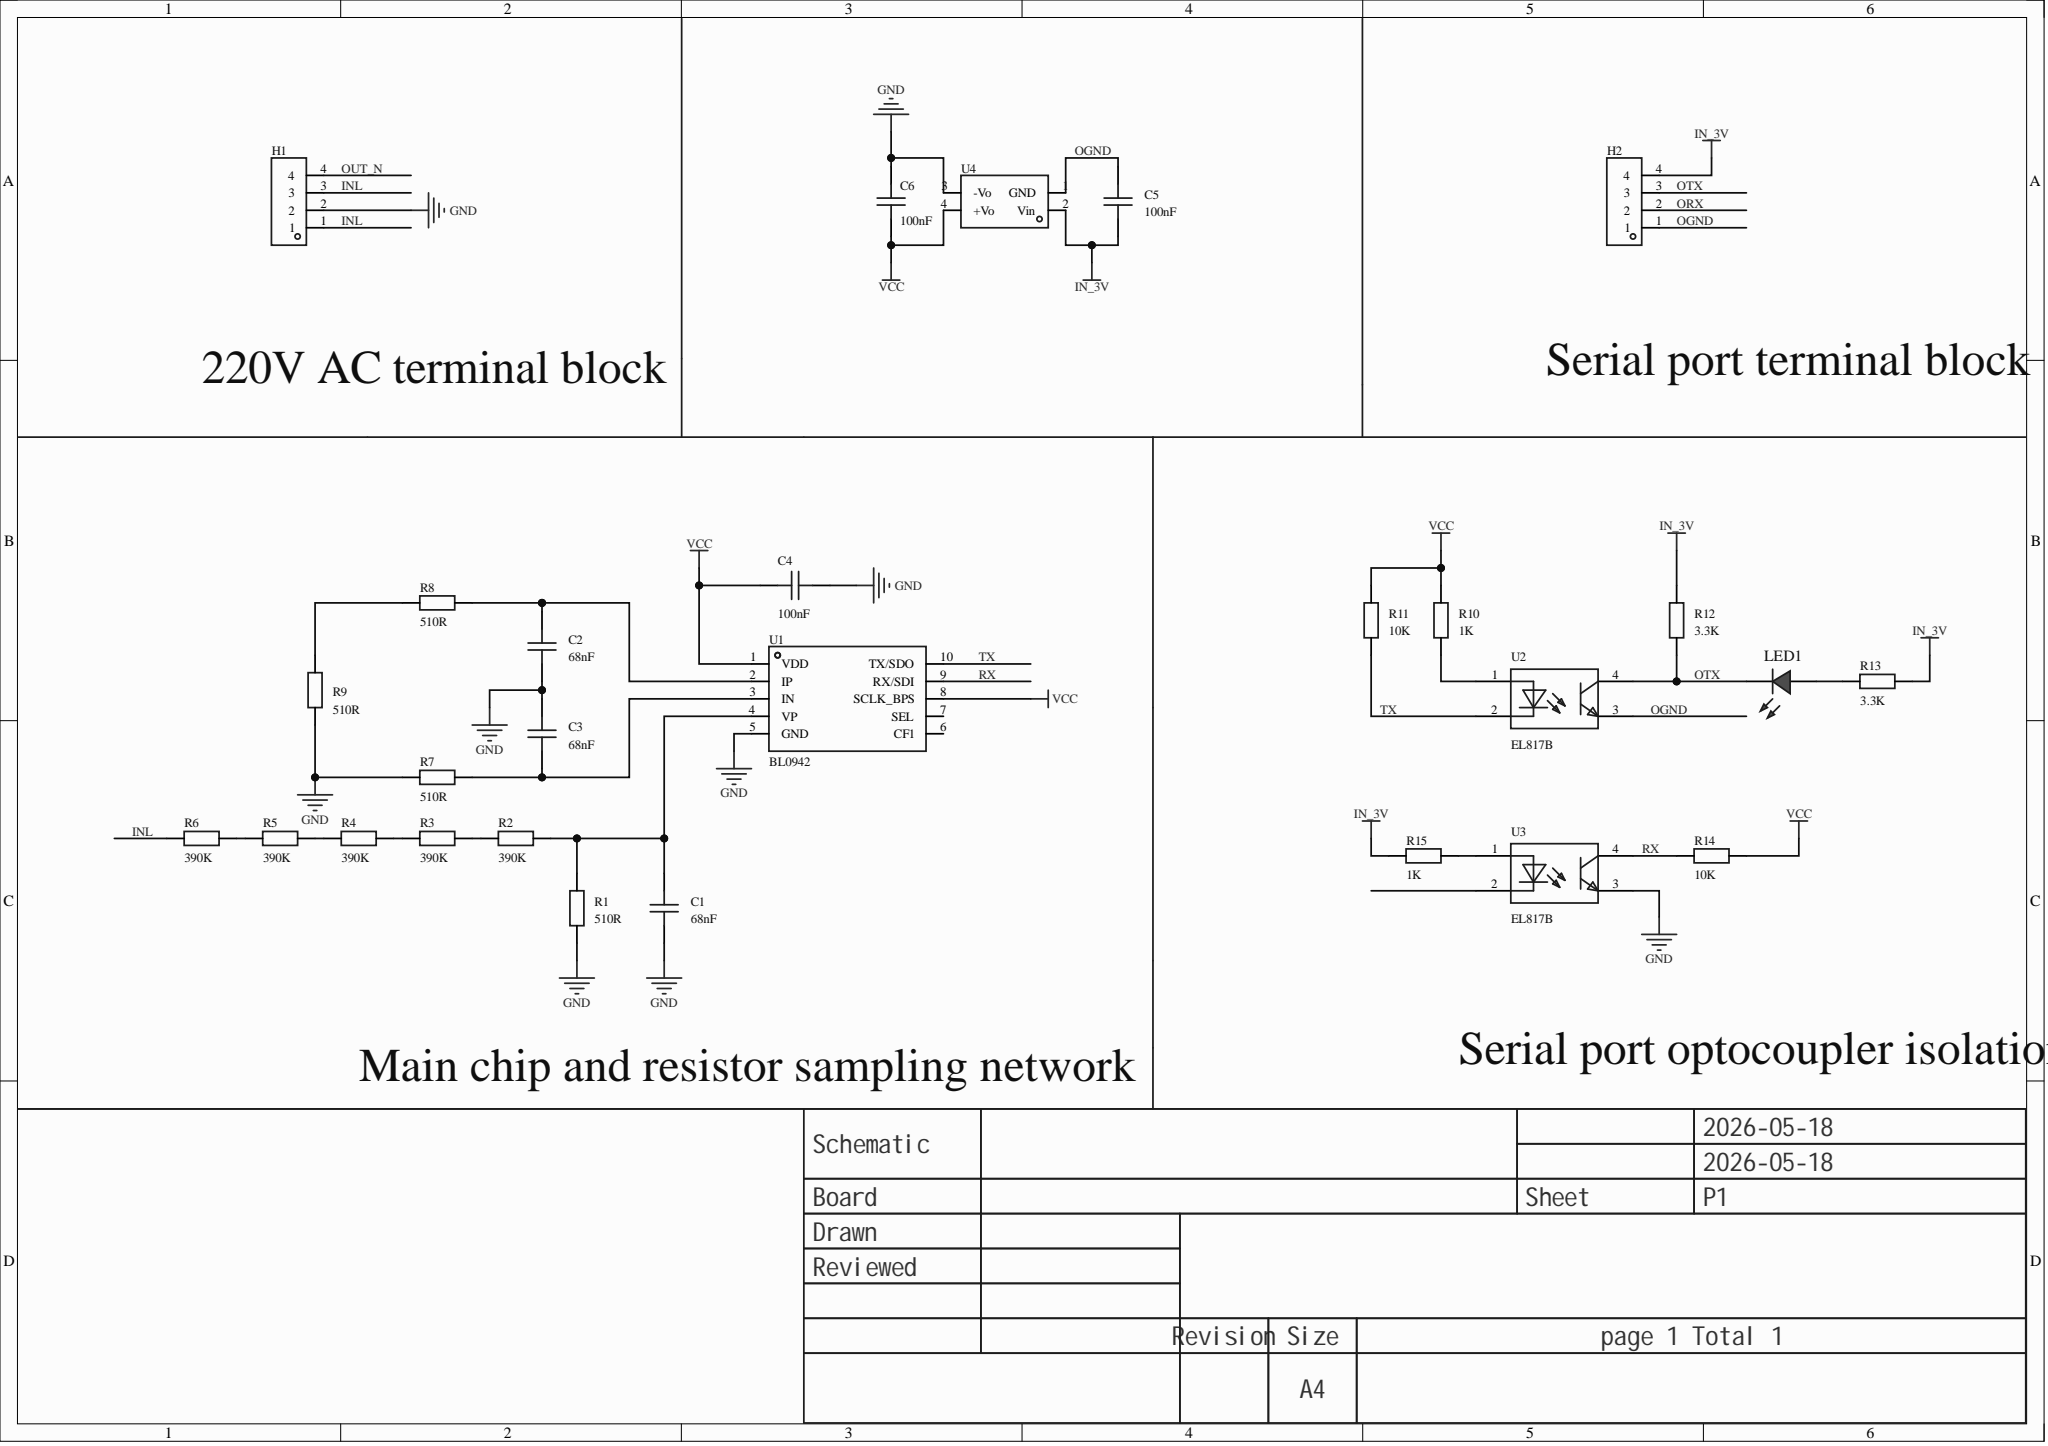Circuit board | Altium Designer | 28 parts | 19 nets
Bill of materials:
Comment,Description,Designator,Footprint,LibRef,Quantity
"68nF","","C1, C2, C3","C0603","CAP_0603","3"
"100nF","","C4, C5, C6","C0603","CAP_0603","3"
"","","H1, H2","HDR-TH_4P-P2.54-V-F","HDR-F_2.54_1x4P","2"
"","","LED1","LED_0603","LED_0603-R","1"
"510R","","R1, R7, R8, R9","R0603","Res_0603","4"
"390K","","R2, R3, R4, R5, R6","R0603","Res_0603","5"
"1K","","R10, R15","R0603","Res_0603","2"
"10K","","R11, R14","R0603","Res_0603","2"
"3.3K","","R12, R13","R0603","Res_0603","2"
"BL0942","BL0942 is an energy metering chip with built-in clock and no calibration needed, for single-phase multifunction meters, smart sockets, smart appliances and similar uses, with high cost performance.","U1","SSOP-10_L4.9-W3.9-P1.00-LS6.0-BL","BL0942_C2837510","1"
"EL817B","","U2, U3","DIP-4_L6.5-W4.6-P2.54-LS7.6-BL","EL817B","2"
"270kHz","","U4","PWRM-TH_B0305S-1WR2","B0305S-1WR2","1"
Netlist (Protel format):
[
C1
C0603
68nF



]
[
C2
C0603
68nF



]
[
C3
C0603
68nF



]
[
C4
C0603
100nF



]
[
C5
C0603
100nF



]
[
C6
C0603
100nF



]
[
H1
HDR-TH_4P-P2.54-V-F




]
[
H2
HDR-TH_4P-P2.54-V-F




]
[
LED1
LED_0603




]
[
R1
R0603
510R



]
[
R2
R0603
390K



]
[
R3
R0603
390K



]
[
R4
R0603
390K



]
[
R5
R0603
390K



]
[
R6
R0603
390K



]
[
R7
R0603
510R



]
[
R8
R0603
510R



]
[
R9
R0603
510R



]
[
R10
R0603
1K



]
[
R11
R0603
10K



]
[
R12
R0603
3.3K



]
[
R13
R0603
3.3K



]
[
R14
R0603
10K



]
[
R15
R0603
1K



]
[
U1
SSOP-10_L4.9-W3.9-P1.00-LS6.0-BL
BL0942



]
[
U2
DIP-4_L6.5-W4.6-P2.54-LS7.6-BL
EL817B



]
[
U3
DIP-4_L6.5-W4.6-P2.54-LS7.6-BL
EL817B



]
[
U4
PWRM-TH_B0305S-1WR2
270kHz



]
(
VCC
C4-2
C6-1
R10-1
R11-1
R14-2
U1-1
U1-8
U4-4
)
(
TX
R11-2
U1-10
U2-2
)
(
RX
R14-1
U1-9
U3-4
)
(
OTX
H2-3
LED1-1
R12-2
U2-4
)
(
OGND
C5-1
H2-1
U2-3
U4-1
)
(
NetR15_2
R15-2
U3-1
)
(
NetR10_2
R10-2
U2-1
)
(
NetR8_2
R8-2
R9-1
)
(
NetR5_2
R5-2
R6-1
)
(
NetR4_2
R4-2
R5-1
)
(
NetR3_2
R3-2
R4-1
)
(
NetR2_2
R2-2
R3-1
)
(
NetLED1_2
LED1-2
R13-1
)
(
NetC3_1
C3-1
R7-1
U1-3
)
(
NetC2_2
C2-2
R8-1
U1-2
)
(
NetC1_2
C1-2
R1-2
R2-1
U1-4
)
(
INL
H1-1
H1-3
R6-2
)
(
IN_3V
C5-2
H2-4
R12-1
R13-2
R15-1
U4-2
)
(
GND
C1-1
C2-1
C3-2
C4-1
C6-2
H1-2
R1-1
R7-2
R9-2
U1-5
U3-3
U4-3
)